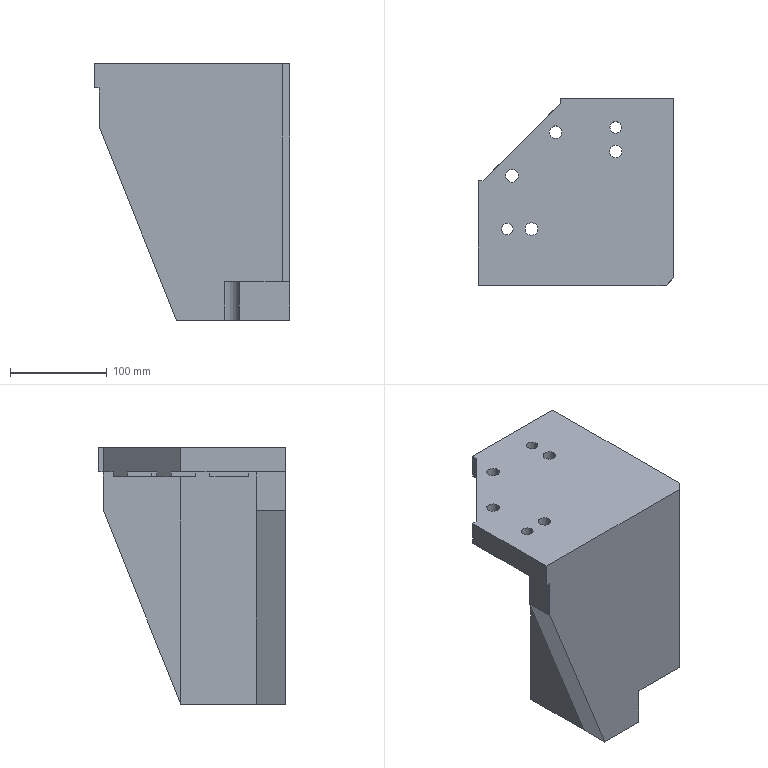Part | NX | features solid 2 | 1 solid | 58 faces | box 202 x 193 x 265 mm | volume 4396749 mm3 | plane 47 | cylinder 11 | commonest cylinder face diameters 13 x4 20 x4 12 x2 30 x1